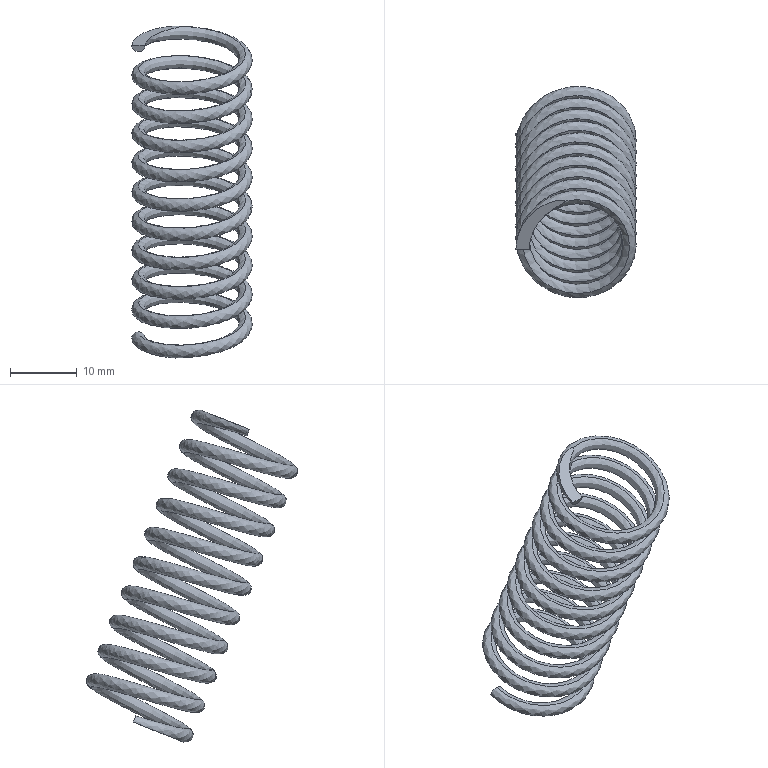Part | STEP file | Ci_cie powierzchni_3 | 1 solid | 6 faces | box 18 x 31.651 x 49.627 mm | volume 1562 mm3 | plane 4 | spline 2